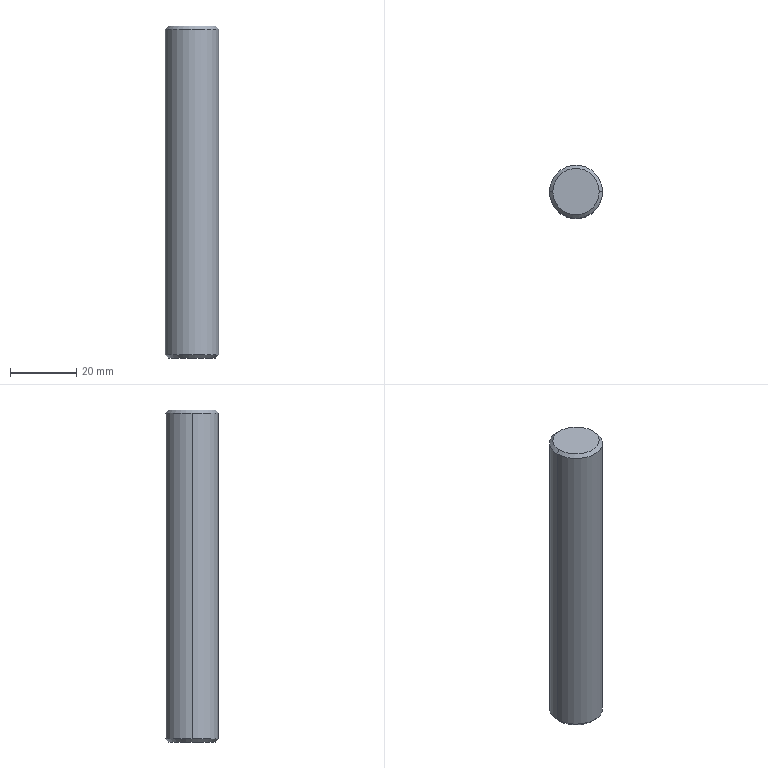Part | STEP file | Foot screw rod | 1 solid | 8 faces | box 16 x 16 x 100 mm | volume 20058 mm3 | cone 4 | cylinder 2 | plane 2 | commonest cylinder face diameters 16 x2
STEP:
#1=CARTESIAN_POINT('',(0.,0.,0.));
#2=DIRECTION('',(0.,0.,1.));
#3=DIRECTION('',(1.,0.,0.));
#4=AXIS2_PLACEMENT_3D('',#1,#2,#3);
#5=CARTESIAN_POINT('',(7.,0.,100.));
#6=VERTEX_POINT('',#5);
#7=CARTESIAN_POINT('',(-7.,0.,100.));
#8=VERTEX_POINT('',#7);
#9=CARTESIAN_POINT('',(0.,0.,100.));
#10=DIRECTION('',(0.,0.,1.));
#11=DIRECTION('',(1.,0.,0.));
#12=AXIS2_PLACEMENT_3D('',#9,#10,#11);
#13=CIRCLE('',#12,7.);
#14=CARTESIAN_POINT('',(0.,0.,100.));
#15=DIRECTION('',(0.,0.,-1.));
#16=DIRECTION('',(-1.,0.,0.));
#17=AXIS2_PLACEMENT_3D('',#14,#15,#16);
#18=CONICAL_SURFACE('',#17,7.,0.7854);
#19=CARTESIAN_POINT('',(3.142,0.));
#20=DIRECTION('',(-1.,0.));
#21=VECTOR('',#20,1.);
#22=LINE('',#19,#21);
#23=(GEOMETRIC_REPRESENTATION_CONTEXT(2)PARAMETRIC_REPRESENTATION_CONTEXT()REPRESENTATION_CONTEXT('',''));
#24=DEFINITIONAL_REPRESENTATION('',(#22),#23);
#25=PCURVE('',#18,#24);
#26=CARTESIAN_POINT('',(0.,0.,100.));
#27=DIRECTION('',(0.,0.,1.));
#28=DIRECTION('',(1.,0.,0.));
#29=AXIS2_PLACEMENT_3D('',#26,#27,#28);
#30=PLANE('',#29);
#31=CARTESIAN_POINT('',(0.,0.));
#32=DIRECTION('',(1.,0.));
#33=AXIS2_PLACEMENT_2D('',#31,#32);
#34=CIRCLE('',#33,7.);
#35=(GEOMETRIC_REPRESENTATION_CONTEXT(2)PARAMETRIC_REPRESENTATION_CONTEXT()REPRESENTATION_CONTEXT('',''));
#36=DEFINITIONAL_REPRESENTATION('',(#34),#35);
#37=PCURVE('',#30,#36);
#38=SURFACE_CURVE('',#13,(#25,#37),.PCURVE_S1.);
#39=EDGE_CURVE('',#6,#8,#38,.T.);
#40=ORIENTED_EDGE('',*,*,#39,.F.);
#41=CARTESIAN_POINT('',(8.,0.,99.));
#42=VERTEX_POINT('',#41);
#43=CARTESIAN_POINT('',(7.,0.,100.));
#44=DIRECTION('',(0.7071,0.,-0.7071));
#45=VECTOR('',#44,1.);
#46=LINE('',#43,#45);
#47=CARTESIAN_POINT('',(3.142,0.));
#48=DIRECTION('',(0.,1.));
#49=VECTOR('',#48,1.);
#50=LINE('',#47,#49);
#51=(GEOMETRIC_REPRESENTATION_CONTEXT(2)PARAMETRIC_REPRESENTATION_CONTEXT()REPRESENTATION_CONTEXT('',''));
#52=DEFINITIONAL_REPRESENTATION('',(#50),#51);
#53=PCURVE('',#18,#52);
#54=CARTESIAN_POINT('',(0.,0.,100.));
#55=DIRECTION('',(0.,0.,-1.));
#56=DIRECTION('',(-1.,0.,0.));
#57=AXIS2_PLACEMENT_3D('',#54,#55,#56);
#58=CONICAL_SURFACE('',#57,7.,0.7854);
#59=CARTESIAN_POINT('',(3.142,0.));
#60=DIRECTION('',(0.,1.));
#61=VECTOR('',#60,1.);
#62=LINE('',#59,#61);
#63=(GEOMETRIC_REPRESENTATION_CONTEXT(2)PARAMETRIC_REPRESENTATION_CONTEXT()REPRESENTATION_CONTEXT('',''));
#64=DEFINITIONAL_REPRESENTATION('',(#62),#63);
#65=PCURVE('',#58,#64);
#66=SURFACE_CURVE('',#46,(#53,#65),.PCURVE_S1.);
#67=EDGE_CURVE('',#6,#42,#66,.T.);
#68=ORIENTED_EDGE('',*,*,#67,.T.);
#69=CARTESIAN_POINT('',(-8.,0.,99.));
#70=VERTEX_POINT('',#69);
#71=CARTESIAN_POINT('',(0.,0.,99.));
#72=DIRECTION('',(0.,0.,-1.));
#73=DIRECTION('',(1.,0.,0.));
#74=AXIS2_PLACEMENT_3D('',#71,#72,#73);
#75=CIRCLE('',#74,8.);
#76=CARTESIAN_POINT('',(-3.142,1.));
#77=DIRECTION('',(1.,0.));
#78=VECTOR('',#77,1.);
#79=LINE('',#76,#78);
#80=(GEOMETRIC_REPRESENTATION_CONTEXT(2)PARAMETRIC_REPRESENTATION_CONTEXT()REPRESENTATION_CONTEXT('',''));
#81=DEFINITIONAL_REPRESENTATION('',(#79),#80);
#82=PCURVE('',#18,#81);
#83=CARTESIAN_POINT('',(0.,0.,100.));
#84=DIRECTION('',(0.,0.,-1.));
#85=DIRECTION('',(-1.,0.,0.));
#86=AXIS2_PLACEMENT_3D('',#83,#84,#85);
#87=CYLINDRICAL_SURFACE('',#86,8.);
#88=CARTESIAN_POINT('',(-3.142,1.));
#89=DIRECTION('',(1.,0.));
#90=VECTOR('',#89,1.);
#91=LINE('',#88,#90);
#92=(GEOMETRIC_REPRESENTATION_CONTEXT(2)PARAMETRIC_REPRESENTATION_CONTEXT()REPRESENTATION_CONTEXT('',''));
#93=DEFINITIONAL_REPRESENTATION('',(#91),#92);
#94=PCURVE('',#87,#93);
#95=SURFACE_CURVE('',#75,(#82,#94),.PCURVE_S1.);
#96=EDGE_CURVE('',#70,#42,#95,.T.);
#97=ORIENTED_EDGE('',*,*,#96,.F.);
#98=CARTESIAN_POINT('',(-7.,0.,100.));
#99=DIRECTION('',(-0.7071,0.,-0.7071));
#100=VECTOR('',#99,1.);
#101=LINE('',#98,#100);
#102=CARTESIAN_POINT('',(0.,0.));
#103=DIRECTION('',(0.,1.));
#104=VECTOR('',#103,1.);
#105=LINE('',#102,#104);
#106=(GEOMETRIC_REPRESENTATION_CONTEXT(2)PARAMETRIC_REPRESENTATION_CONTEXT()REPRESENTATION_CONTEXT('',''));
#107=DEFINITIONAL_REPRESENTATION('',(#105),#106);
#108=PCURVE('',#18,#107);
#109=CARTESIAN_POINT('',(6.283,0.));
#110=DIRECTION('',(0.,1.));
#111=VECTOR('',#110,1.);
#112=LINE('',#109,#111);
#113=(GEOMETRIC_REPRESENTATION_CONTEXT(2)PARAMETRIC_REPRESENTATION_CONTEXT()REPRESENTATION_CONTEXT('',''));
#114=DEFINITIONAL_REPRESENTATION('',(#112),#113);
#115=PCURVE('',#58,#114);
#116=SURFACE_CURVE('',#101,(#108,#115),.PCURVE_S1.);
#117=EDGE_CURVE('',#8,#70,#116,.T.);
#118=ORIENTED_EDGE('',*,*,#117,.F.);
#119=EDGE_LOOP('',(#40,#68,#97,#118));
#120=FACE_BOUND('',#119,.T.);
#121=ADVANCED_FACE('',(#120),#18,.T.);
#122=CARTESIAN_POINT('',(-7.,0.,0.));
#123=VERTEX_POINT('',#122);
#124=CARTESIAN_POINT('',(7.,0.,0.));
#125=VERTEX_POINT('',#124);
#126=CARTESIAN_POINT('',(0.,0.,0.));
#127=DIRECTION('',(0.,0.,-1.));
#128=DIRECTION('',(1.,0.,0.));
#129=AXIS2_PLACEMENT_3D('',#126,#127,#128);
#130=CIRCLE('',#129,7.);
#131=CARTESIAN_POINT('',(0.,0.,1.));
#132=DIRECTION('',(0.,0.,1.));
#133=DIRECTION('',(1.,0.,0.));
#134=AXIS2_PLACEMENT_3D('',#131,#132,#133);
#135=CONICAL_SURFACE('',#134,8.,0.7854);
#136=CARTESIAN_POINT('',(6.283,-1.));
#137=DIRECTION('',(-1.,0.));
#138=VECTOR('',#137,1.);
#139=LINE('',#136,#138);
#140=(GEOMETRIC_REPRESENTATION_CONTEXT(2)PARAMETRIC_REPRESENTATION_CONTEXT()REPRESENTATION_CONTEXT('',''));
#141=DEFINITIONAL_REPRESENTATION('',(#139),#140);
#142=PCURVE('',#135,#141);
#143=CARTESIAN_POINT('',(0.,0.,0.));
#144=DIRECTION('',(0.,0.,1.));
#145=DIRECTION('',(1.,0.,0.));
#146=AXIS2_PLACEMENT_3D('',#143,#144,#145);
#147=PLANE('',#146);
#148=CARTESIAN_POINT('',(7.,0.));
#149=CARTESIAN_POINT('',(7.,-12.124));
#150=CARTESIAN_POINT('',(-3.5,-6.062));
#151=CARTESIAN_POINT('',(-14.,0.));
#152=CARTESIAN_POINT('',(-3.5,6.062));
#153=CARTESIAN_POINT('',(7.,12.124));
#154=CARTESIAN_POINT('',(7.,0.));
#155=(BOUNDED_CURVE()B_SPLINE_CURVE(2,(#148,#149,#150,#151,#152,#153,#154),.UNSPECIFIED.,.T.,.F.)B_SPLINE_CURVE_WITH_KNOTS((1,2,2,2,2,1),(-2.094,0.,2.094,4.189,6.283,8.378),.UNSPECIFIED.)CURVE()GEOMETRIC_REPRESENTATION_ITEM()RATIONAL_B_SPLINE_CURVE((1.,0.5,1.,0.5,1.,0.5,1.))REPRESENTATION_ITEM(''));
#156=(GEOMETRIC_REPRESENTATION_CONTEXT(2)PARAMETRIC_REPRESENTATION_CONTEXT()REPRESENTATION_CONTEXT('',''));
#157=DEFINITIONAL_REPRESENTATION('',(#155),#156);
#158=PCURVE('',#147,#157);
#159=SURFACE_CURVE('',#130,(#142,#158),.PCURVE_S1.);
#160=EDGE_CURVE('',#123,#125,#159,.T.);
#161=ORIENTED_EDGE('',*,*,#160,.F.);
#162=CARTESIAN_POINT('',(-8.,0.,1.));
#163=VERTEX_POINT('',#162);
#164=CARTESIAN_POINT('',(-8.,0.,1.));
#165=DIRECTION('',(-0.7071,0.,0.7071));
#166=VECTOR('',#165,1.);
#167=LINE('',#164,#166);
#168=CARTESIAN_POINT('',(3.142,0.));
#169=DIRECTION('',(0.,1.));
#170=VECTOR('',#169,1.);
#171=LINE('',#168,#170);
#172=(GEOMETRIC_REPRESENTATION_CONTEXT(2)PARAMETRIC_REPRESENTATION_CONTEXT()REPRESENTATION_CONTEXT('',''));
#173=DEFINITIONAL_REPRESENTATION('',(#171),#172);
#174=PCURVE('',#135,#173);
#175=CARTESIAN_POINT('',(0.,0.,1.));
#176=DIRECTION('',(0.,0.,1.));
#177=DIRECTION('',(1.,0.,0.));
#178=AXIS2_PLACEMENT_3D('',#175,#176,#177);
#179=CONICAL_SURFACE('',#178,8.,0.7854);
#180=CARTESIAN_POINT('',(3.142,0.));
#181=DIRECTION('',(0.,1.));
#182=VECTOR('',#181,1.);
#183=LINE('',#180,#182);
#184=(GEOMETRIC_REPRESENTATION_CONTEXT(2)PARAMETRIC_REPRESENTATION_CONTEXT()REPRESENTATION_CONTEXT('',''));
#185=DEFINITIONAL_REPRESENTATION('',(#183),#184);
#186=PCURVE('',#179,#185);
#187=SURFACE_CURVE('',#167,(#174,#186),.PCURVE_S1.);
#188=EDGE_CURVE('',#123,#163,#187,.T.);
#189=ORIENTED_EDGE('',*,*,#188,.T.);
#190=CARTESIAN_POINT('',(8.,0.,1.));
#191=VERTEX_POINT('',#190);
#192=CARTESIAN_POINT('',(0.,0.,1.));
#193=DIRECTION('',(0.,0.,1.));
#194=DIRECTION('',(1.,0.,0.));
#195=AXIS2_PLACEMENT_3D('',#192,#193,#194);
#196=CIRCLE('',#195,8.);
#197=CARTESIAN_POINT('',(0.,0.));
#198=DIRECTION('',(1.,0.));
#199=VECTOR('',#198,1.);
#200=LINE('',#197,#199);
#201=(GEOMETRIC_REPRESENTATION_CONTEXT(2)PARAMETRIC_REPRESENTATION_CONTEXT()REPRESENTATION_CONTEXT('',''));
#202=DEFINITIONAL_REPRESENTATION('',(#200),#201);
#203=PCURVE('',#135,#202);
#204=CARTESIAN_POINT('',(3.142,99.));
#205=DIRECTION('',(-1.,0.));
#206=VECTOR('',#205,1.);
#207=LINE('',#204,#206);
#208=(GEOMETRIC_REPRESENTATION_CONTEXT(2)PARAMETRIC_REPRESENTATION_CONTEXT()REPRESENTATION_CONTEXT('',''));
#209=DEFINITIONAL_REPRESENTATION('',(#207),#208);
#210=PCURVE('',#87,#209);
#211=SURFACE_CURVE('',#196,(#203,#210),.PCURVE_S1.);
#212=EDGE_CURVE('',#191,#163,#211,.T.);
#213=ORIENTED_EDGE('',*,*,#212,.F.);
#214=CARTESIAN_POINT('',(8.,0.,1.));
#215=DIRECTION('',(0.7071,0.,0.7071));
#216=VECTOR('',#215,1.);
#217=LINE('',#214,#216);
#218=CARTESIAN_POINT('',(0.,0.));
#219=DIRECTION('',(0.,1.));
#220=VECTOR('',#219,1.);
#221=LINE('',#218,#220);
#222=(GEOMETRIC_REPRESENTATION_CONTEXT(2)PARAMETRIC_REPRESENTATION_CONTEXT()REPRESENTATION_CONTEXT('',''));
#223=DEFINITIONAL_REPRESENTATION('',(#221),#222);
#224=PCURVE('',#135,#223);
#225=CARTESIAN_POINT('',(6.283,0.));
#226=DIRECTION('',(0.,1.));
#227=VECTOR('',#226,1.);
#228=LINE('',#225,#227);
#229=(GEOMETRIC_REPRESENTATION_CONTEXT(2)PARAMETRIC_REPRESENTATION_CONTEXT()REPRESENTATION_CONTEXT('',''));
#230=DEFINITIONAL_REPRESENTATION('',(#228),#229);
#231=PCURVE('',#179,#230);
#232=SURFACE_CURVE('',#217,(#224,#231),.PCURVE_S1.);
#233=EDGE_CURVE('',#125,#191,#232,.T.);
#234=ORIENTED_EDGE('',*,*,#233,.F.);
#235=EDGE_LOOP('',(#161,#189,#213,#234));
#236=FACE_BOUND('',#235,.T.);
#237=ADVANCED_FACE('',(#236),#135,.T.);
#238=ORIENTED_EDGE('',*,*,#96,.T.);
#239=CARTESIAN_POINT('',(8.,0.,100.));
#240=DIRECTION('',(0.,0.,-1.));
#241=VECTOR('',#240,1.);
#242=LINE('',#239,#241);
#243=CARTESIAN_POINT('',(3.142,0.));
#244=DIRECTION('',(0.,1.));
#245=VECTOR('',#244,1.);
#246=LINE('',#243,#245);
#247=(GEOMETRIC_REPRESENTATION_CONTEXT(2)PARAMETRIC_REPRESENTATION_CONTEXT()REPRESENTATION_CONTEXT('',''));
#248=DEFINITIONAL_REPRESENTATION('',(#246),#247);
#249=PCURVE('',#87,#248);
#250=CARTESIAN_POINT('',(0.,0.,100.));
#251=DIRECTION('',(0.,0.,-1.));
#252=DIRECTION('',(-1.,0.,0.));
#253=AXIS2_PLACEMENT_3D('',#250,#251,#252);
#254=CYLINDRICAL_SURFACE('',#253,8.);
#255=CARTESIAN_POINT('',(3.142,0.));
#256=DIRECTION('',(0.,1.));
#257=VECTOR('',#256,1.);
#258=LINE('',#255,#257);
#259=(GEOMETRIC_REPRESENTATION_CONTEXT(2)PARAMETRIC_REPRESENTATION_CONTEXT()REPRESENTATION_CONTEXT('',''));
#260=DEFINITIONAL_REPRESENTATION('',(#258),#259);
#261=PCURVE('',#254,#260);
#262=SURFACE_CURVE('',#242,(#249,#261),.PCURVE_S1.);
#263=EDGE_CURVE('',#42,#191,#262,.T.);
#264=ORIENTED_EDGE('',*,*,#263,.T.);
#265=ORIENTED_EDGE('',*,*,#212,.T.);
#266=CARTESIAN_POINT('',(-8.,0.,100.));
#267=DIRECTION('',(0.,0.,-1.));
#268=VECTOR('',#267,1.);
#269=LINE('',#266,#268);
#270=CARTESIAN_POINT('',(0.,0.));
#271=DIRECTION('',(0.,1.));
#272=VECTOR('',#271,1.);
#273=LINE('',#270,#272);
#274=(GEOMETRIC_REPRESENTATION_CONTEXT(2)PARAMETRIC_REPRESENTATION_CONTEXT()REPRESENTATION_CONTEXT('',''));
#275=DEFINITIONAL_REPRESENTATION('',(#273),#274);
#276=PCURVE('',#87,#275);
#277=CARTESIAN_POINT('',(6.283,0.));
#278=DIRECTION('',(0.,1.));
#279=VECTOR('',#278,1.);
#280=LINE('',#277,#279);
#281=(GEOMETRIC_REPRESENTATION_CONTEXT(2)PARAMETRIC_REPRESENTATION_CONTEXT()REPRESENTATION_CONTEXT('',''));
#282=DEFINITIONAL_REPRESENTATION('',(#280),#281);
#283=PCURVE('',#254,#282);
#284=SURFACE_CURVE('',#269,(#276,#283),.PCURVE_S1.);
#285=EDGE_CURVE('',#70,#163,#284,.T.);
#286=ORIENTED_EDGE('',*,*,#285,.F.);
#287=EDGE_LOOP('',(#238,#264,#265,#286));
#288=FACE_BOUND('',#287,.T.);
#289=ADVANCED_FACE('',(#288),#87,.T.);
#290=ORIENTED_EDGE('',*,*,#263,.F.);
#291=CARTESIAN_POINT('',(0.,0.,99.));
#292=DIRECTION('',(0.,0.,-1.));
#293=DIRECTION('',(1.,0.,0.));
#294=AXIS2_PLACEMENT_3D('',#291,#292,#293);
#295=CIRCLE('',#294,8.);
#296=CARTESIAN_POINT('',(3.142,1.));
#297=DIRECTION('',(1.,0.));
#298=VECTOR('',#297,1.);
#299=LINE('',#296,#298);
#300=(GEOMETRIC_REPRESENTATION_CONTEXT(2)PARAMETRIC_REPRESENTATION_CONTEXT()REPRESENTATION_CONTEXT('',''));
#301=DEFINITIONAL_REPRESENTATION('',(#299),#300);
#302=PCURVE('',#254,#301);
#303=CARTESIAN_POINT('',(3.142,1.));
#304=DIRECTION('',(1.,0.));
#305=VECTOR('',#304,1.);
#306=LINE('',#303,#305);
#307=(GEOMETRIC_REPRESENTATION_CONTEXT(2)PARAMETRIC_REPRESENTATION_CONTEXT()REPRESENTATION_CONTEXT('',''));
#308=DEFINITIONAL_REPRESENTATION('',(#306),#307);
#309=PCURVE('',#58,#308);
#310=SURFACE_CURVE('',#295,(#302,#309),.PCURVE_S1.);
#311=EDGE_CURVE('',#42,#70,#310,.T.);
#312=ORIENTED_EDGE('',*,*,#311,.T.);
#313=ORIENTED_EDGE('',*,*,#285,.T.);
#314=CARTESIAN_POINT('',(0.,0.,1.));
#315=DIRECTION('',(0.,0.,1.));
#316=DIRECTION('',(1.,0.,0.));
#317=AXIS2_PLACEMENT_3D('',#314,#315,#316);
#318=CIRCLE('',#317,8.);
#319=CARTESIAN_POINT('',(9.425,99.));
#320=DIRECTION('',(-1.,0.));
#321=VECTOR('',#320,1.);
#322=LINE('',#319,#321);
#323=(GEOMETRIC_REPRESENTATION_CONTEXT(2)PARAMETRIC_REPRESENTATION_CONTEXT()REPRESENTATION_CONTEXT('',''));
#324=DEFINITIONAL_REPRESENTATION('',(#322),#323);
#325=PCURVE('',#254,#324);
#326=CARTESIAN_POINT('',(0.,0.));
#327=DIRECTION('',(1.,0.));
#328=VECTOR('',#327,1.);
#329=LINE('',#326,#328);
#330=(GEOMETRIC_REPRESENTATION_CONTEXT(2)PARAMETRIC_REPRESENTATION_CONTEXT()REPRESENTATION_CONTEXT('',''));
#331=DEFINITIONAL_REPRESENTATION('',(#329),#330);
#332=PCURVE('',#179,#331);
#333=SURFACE_CURVE('',#318,(#325,#332),.PCURVE_S1.);
#334=EDGE_CURVE('',#163,#191,#333,.T.);
#335=ORIENTED_EDGE('',*,*,#334,.T.);
#336=EDGE_LOOP('',(#290,#312,#313,#335));
#337=FACE_BOUND('',#336,.T.);
#338=ADVANCED_FACE('',(#337),#254,.T.);
#339=CARTESIAN_POINT('',(0.,0.,100.));
#340=DIRECTION('',(0.,0.,1.));
#341=DIRECTION('',(1.,0.,0.));
#342=AXIS2_PLACEMENT_3D('',#339,#340,#341);
#343=CIRCLE('',#342,7.);
#344=CARTESIAN_POINT('',(0.,0.));
#345=DIRECTION('',(1.,0.));
#346=AXIS2_PLACEMENT_2D('',#344,#345);
#347=CIRCLE('',#346,7.);
#348=(GEOMETRIC_REPRESENTATION_CONTEXT(2)PARAMETRIC_REPRESENTATION_CONTEXT()REPRESENTATION_CONTEXT('',''));
#349=DEFINITIONAL_REPRESENTATION('',(#347),#348);
#350=PCURVE('',#30,#349);
#351=CARTESIAN_POINT('',(9.425,0.));
#352=DIRECTION('',(-1.,0.));
#353=VECTOR('',#352,1.);
#354=LINE('',#351,#353);
#355=(GEOMETRIC_REPRESENTATION_CONTEXT(2)PARAMETRIC_REPRESENTATION_CONTEXT()REPRESENTATION_CONTEXT('',''));
#356=DEFINITIONAL_REPRESENTATION('',(#354),#355);
#357=PCURVE('',#58,#356);
#358=SURFACE_CURVE('',#343,(#350,#357),.PCURVE_S1.);
#359=EDGE_CURVE('',#8,#6,#358,.T.);
#360=ORIENTED_EDGE('',*,*,#359,.T.);
#361=ORIENTED_EDGE('',*,*,#39,.T.);
#362=EDGE_LOOP('',(#360,#361));
#363=FACE_BOUND('',#362,.T.);
#364=ADVANCED_FACE('',(#363),#30,.T.);
#365=CARTESIAN_POINT('',(0.,0.,0.));
#366=DIRECTION('',(0.,0.,-1.));
#367=DIRECTION('',(1.,0.,0.));
#368=AXIS2_PLACEMENT_3D('',#365,#366,#367);
#369=CIRCLE('',#368,7.);
#370=CARTESIAN_POINT('',(7.,0.));
#371=CARTESIAN_POINT('',(7.,-12.124));
#372=CARTESIAN_POINT('',(-3.5,-6.062));
#373=CARTESIAN_POINT('',(-14.,0.));
#374=CARTESIAN_POINT('',(-3.5,6.062));
#375=CARTESIAN_POINT('',(7.,12.124));
#376=CARTESIAN_POINT('',(7.,0.));
#377=(BOUNDED_CURVE()B_SPLINE_CURVE(2,(#370,#371,#372,#373,#374,#375,#376),.UNSPECIFIED.,.T.,.F.)B_SPLINE_CURVE_WITH_KNOTS((1,2,2,2,2,1),(-2.094,0.,2.094,4.189,6.283,8.378),.UNSPECIFIED.)CURVE()GEOMETRIC_REPRESENTATION_ITEM()RATIONAL_B_SPLINE_CURVE((1.,0.5,1.,0.5,1.,0.5,1.))REPRESENTATION_ITEM(''));
#378=(GEOMETRIC_REPRESENTATION_CONTEXT(2)PARAMETRIC_REPRESENTATION_CONTEXT()REPRESENTATION_CONTEXT('',''));
#379=DEFINITIONAL_REPRESENTATION('',(#377),#378);
#380=PCURVE('',#147,#379);
#381=CARTESIAN_POINT('',(6.283,-1.));
#382=DIRECTION('',(-1.,0.));
#383=VECTOR('',#382,1.);
#384=LINE('',#381,#383);
#385=(GEOMETRIC_REPRESENTATION_CONTEXT(2)PARAMETRIC_REPRESENTATION_CONTEXT()REPRESENTATION_CONTEXT('',''));
#386=DEFINITIONAL_REPRESENTATION('',(#384),#385);
#387=PCURVE('',#179,#386);
#388=SURFACE_CURVE('',#369,(#380,#387),.PCURVE_S1.);
#389=EDGE_CURVE('',#125,#123,#388,.T.);
#390=ORIENTED_EDGE('',*,*,#389,.T.);
#391=ORIENTED_EDGE('',*,*,#160,.T.);
#392=EDGE_LOOP('',(#390,#391));
#393=FACE_BOUND('',#392,.T.);
#394=ADVANCED_FACE('',(#393),#147,.F.);
#395=ORIENTED_EDGE('',*,*,#188,.F.);
#396=ORIENTED_EDGE('',*,*,#389,.F.);
#397=ORIENTED_EDGE('',*,*,#233,.T.);
#398=ORIENTED_EDGE('',*,*,#334,.F.);
#399=EDGE_LOOP('',(#395,#396,#397,#398));
#400=FACE_BOUND('',#399,.T.);
#401=ADVANCED_FACE('',(#400),#179,.T.);
#402=ORIENTED_EDGE('',*,*,#67,.F.);
#403=ORIENTED_EDGE('',*,*,#359,.F.);
#404=ORIENTED_EDGE('',*,*,#117,.T.);
#405=ORIENTED_EDGE('',*,*,#311,.F.);
#406=EDGE_LOOP('',(#402,#403,#404,#405));
#407=FACE_BOUND('',#406,.T.);
#408=ADVANCED_FACE('',(#407),#58,.T.);
#409=CLOSED_SHELL('',(#121,#237,#289,#338,#364,#394,#401,#408));
#410=MANIFOLD_SOLID_BREP('',#409);
#411=(LENGTH_UNIT()NAMED_UNIT(*)SI_UNIT(.MILLI.,.METRE.));
#412=UNCERTAINTY_MEASURE_WITH_UNIT(LENGTH_MEASURE(0.0000001),#411,'','');
#413=(NAMED_UNIT(*)PLANE_ANGLE_UNIT()SI_UNIT($,.RADIAN.));
#414=(NAMED_UNIT(*)SI_UNIT($,.STERADIAN.)SOLID_ANGLE_UNIT());
#415=(GEOMETRIC_REPRESENTATION_CONTEXT(3)GLOBAL_UNCERTAINTY_ASSIGNED_CONTEXT((#412))GLOBAL_UNIT_ASSIGNED_CONTEXT((#411,#413,#414))REPRESENTATION_CONTEXT('',''));
#416=ADVANCED_BREP_SHAPE_REPRESENTATION('',(#4,#410),#415);